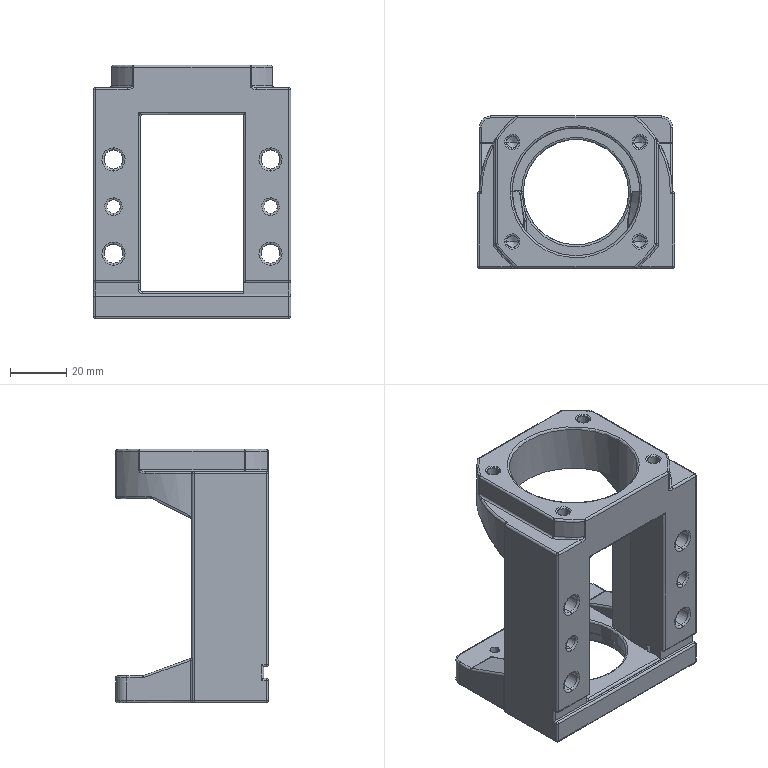Part | STEP file | MJ45 motor base fixing | 1 solid | 336 faces | box 70.4 x 54.4 x 90.4 mm | volume 105657 mm3 | cylinder 135 | spline 129 | plane 42 | cone 30 | commonest cylinder face diameters 1.44 x83 3.44 x8 4.08 x8 6.8 x8 11.2 x8 4.8 x4